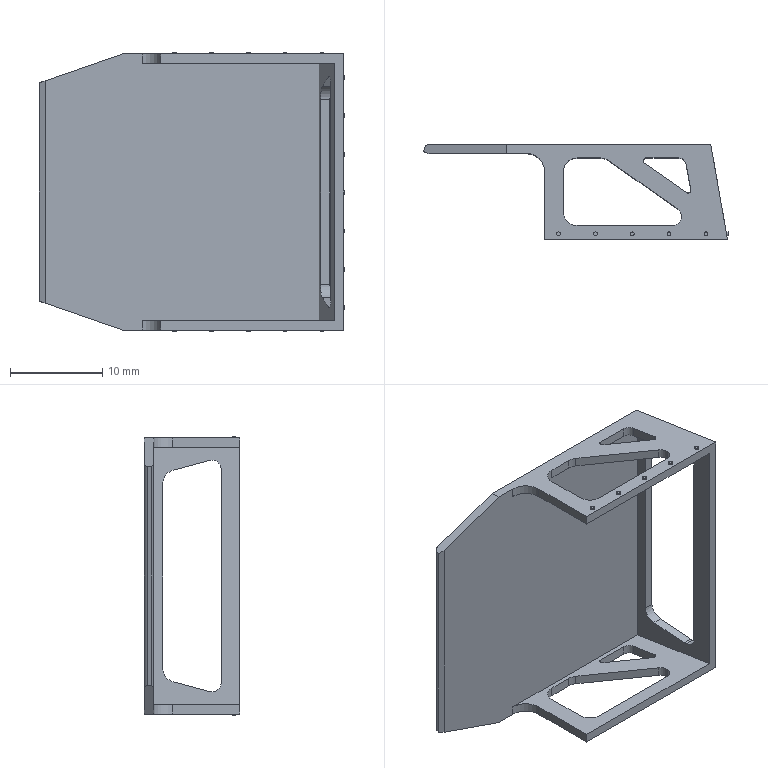Part | SolidWorks | features ICE 5, Extrusion 1, MirrorPattern 1, Shell 1 | 1 solid | 110 faces | box 33.181 x 10.34 x 30.4 mm | volume 1217 mm3 | cylinder 60 | plane 50 | commonest cylinder face diameters 0.4 x34 3 x8 2 x7 0.6 x6 1.72 x2 4 x2